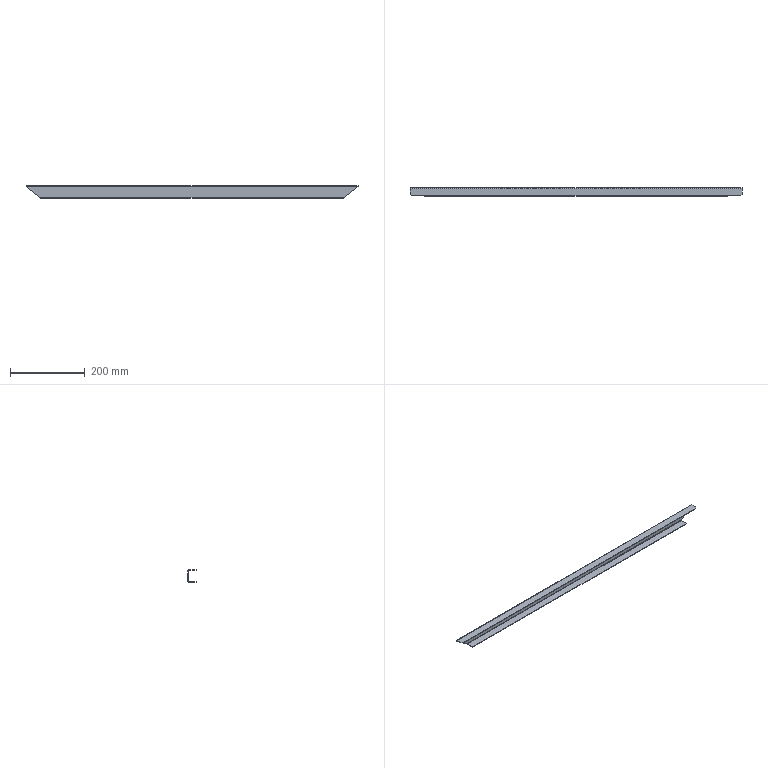Part | STEP file | b-017 | 1 solid | 32 faces | box 890 x 21.5 x 33 mm | volume 91588 mm3 | plane 20 | spline 8 | cylinder 4 | commonest cylinder face diameters 1.473 x2 4.473 x2